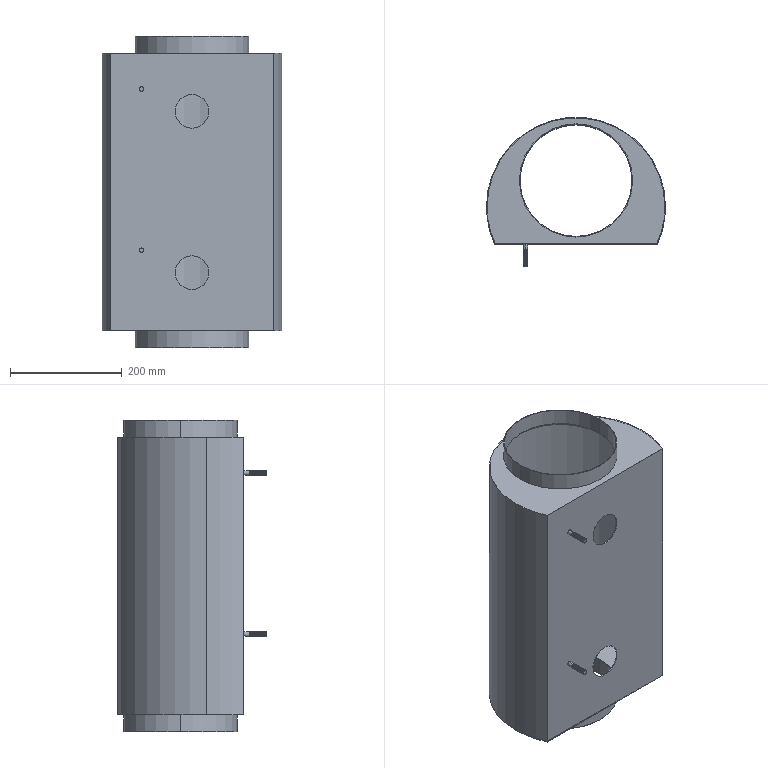Part | SolidWorks | features ICE 7, SweepThread 2, Extrusion 1, Shell 1 | 1 solid | 162 faces | box 320 x 266 x 556 mm | volume 661676 mm3 | cylinder 142 | plane 14 | spline 6 | commonest cylinder face diameters 8 x124 60 x4 200 x4 202.4 x4 317.6 x3 320 x3